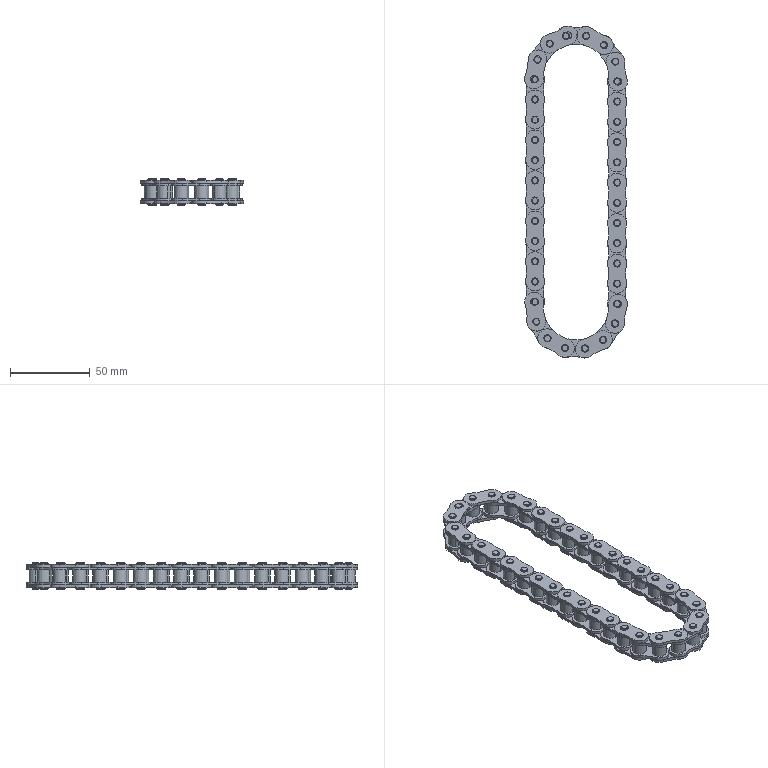Part | SolidWorks | features Boss 3, CurvePattern 2, Chamfer 1, CompositeCurve 1, Extrusion 1, MirrorPattern 1, MirrorSolid 1 | 54 solids | 1080 faces | box 64.757 x 208.466 x 16.625 mm | volume 48801 mm3 | cylinder 720 | plane 216 | cone 144 | commonest cylinder face diameters 4.45 x288 11.81 x216 57.066 x144 8.51 x72